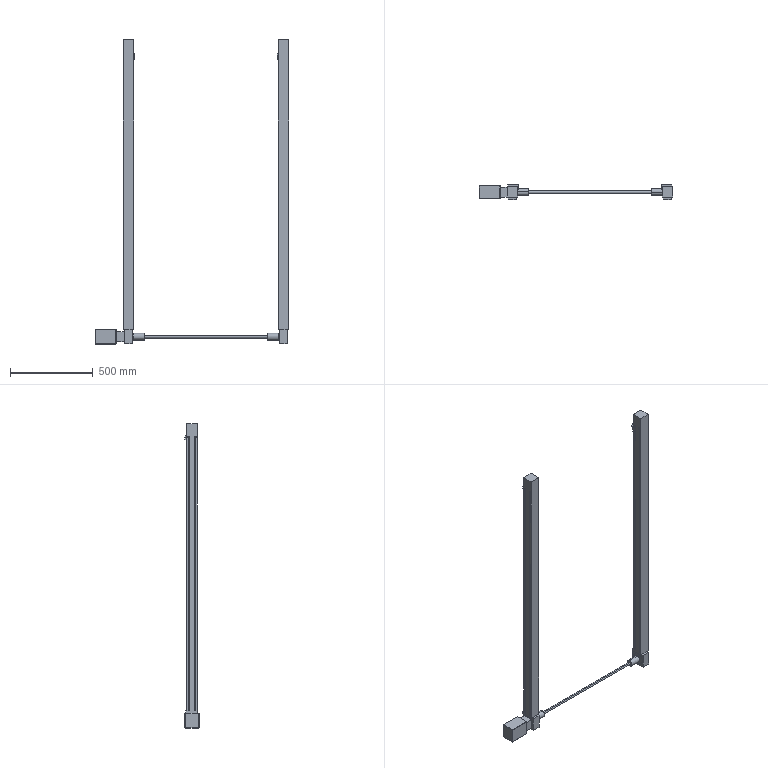Part | SolidWorks | 8 solids | 264 faces | box 1167 x 88 x 1837 mm | volume 15808728 mm3 | plane 214 | cylinder 50 | commonest cylinder face diameters 8 x16 16 x12 5.5 x8 73 x6 40 x4 6 x2